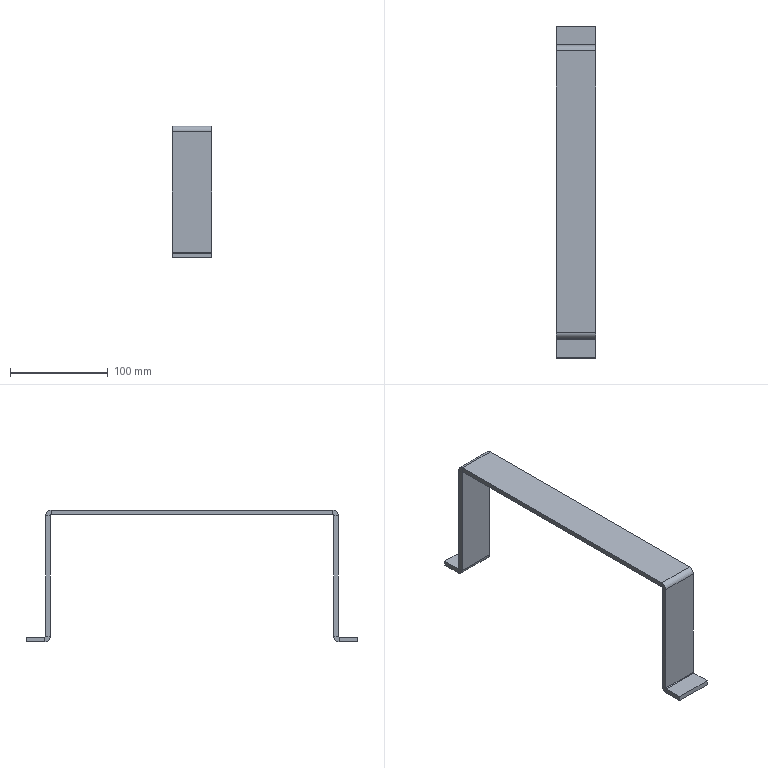Part | SolidWorks | features EdgeFlange 2, FlatPattern 1, SMBaseFlange 1, SheetMetal 1 | 1 solid | 38 faces | box 40 x 340 x 135 mm | volume 118889 mm3 | plane 30 | cylinder 8 | commonest cylinder face diameters 1.473 x4 11.473 x4
STEP:
#1=CARTESIAN_POINT('',(20.,-150.,-5.737));
#2=VERTEX_POINT('',#1);
#3=CARTESIAN_POINT('',(20.,-150.,-129.263));
#4=VERTEX_POINT('',#3);
#5=CARTESIAN_POINT('',(20.,-150.,-5.));
#6=DIRECTION('',(0.,0.,-1.));
#7=VECTOR('',#6,1000.);
#8=LINE('',#5,#7);
#9=EDGE_CURVE('',#2,#4,#8,.T.);
#10=ORIENTED_EDGE('',*,*,#9,.T.);
#11=CARTESIAN_POINT('',(20.,-145.,-129.263));
#12=VERTEX_POINT('',#11);
#13=CARTESIAN_POINT('',(20.,-150.,-129.263));
#14=DIRECTION('',(0.,1.,0.));
#15=VECTOR('',#14,1000.);
#16=LINE('',#13,#15);
#17=EDGE_CURVE('',#4,#12,#16,.T.);
#18=ORIENTED_EDGE('',*,*,#17,.T.);
#19=CARTESIAN_POINT('',(20.,-145.,-5.737));
#20=VERTEX_POINT('',#19);
#21=CARTESIAN_POINT('',(20.,-145.,0.));
#22=DIRECTION('',(0.,0.,-1.));
#23=VECTOR('',#22,1000.);
#24=LINE('',#21,#23);
#25=EDGE_CURVE('',#20,#12,#24,.T.);
#26=ORIENTED_EDGE('',*,*,#25,.F.);
#27=CARTESIAN_POINT('',(20.,-150.,-5.737));
#28=DIRECTION('',(0.,-1.,0.));
#29=VECTOR('',#28,1000.);
#30=LINE('',#27,#29);
#31=EDGE_CURVE('',#20,#2,#30,.T.);
#32=ORIENTED_EDGE('',*,*,#31,.T.);
#33=EDGE_LOOP('',(#10,#18,#26,#32));
#34=FACE_OUTER_BOUND('',#33,.T.);
#35=CARTESIAN_POINT('',(20.,-150.,-5.));
#36=DIRECTION('',(1.,0.,0.));
#37=DIRECTION('',(0.,0.,-1.));
#38=AXIS2_PLACEMENT_3D('',#35,#36,#37);
#39=PLANE('',#38);
#40=ADVANCED_FACE('',(#34),#39,.T.);
#41=CARTESIAN_POINT('',(-20.,-150.,-129.263));
#42=VERTEX_POINT('',#41);
#43=CARTESIAN_POINT('',(20.,-150.,-129.263));
#44=DIRECTION('',(-1.,0.,0.));
#45=VECTOR('',#44,1000.);
#46=LINE('',#43,#45);
#47=EDGE_CURVE('',#4,#42,#46,.T.);
#48=ORIENTED_EDGE('',*,*,#47,.F.);
#49=ORIENTED_EDGE('',*,*,#9,.F.);
#50=CARTESIAN_POINT('',(-20.,-150.,-5.737));
#51=VERTEX_POINT('',#50);
#52=CARTESIAN_POINT('',(20.,-150.,-5.737));
#53=DIRECTION('',(1.,0.,0.));
#54=VECTOR('',#53,1000.);
#55=LINE('',#52,#54);
#56=EDGE_CURVE('',#51,#2,#55,.T.);
#57=ORIENTED_EDGE('',*,*,#56,.F.);
#58=CARTESIAN_POINT('',(-20.,-150.,-135.));
#59=DIRECTION('',(0.,0.,1.));
#60=VECTOR('',#59,1000.);
#61=LINE('',#58,#60);
#62=EDGE_CURVE('',#42,#51,#61,.T.);
#63=ORIENTED_EDGE('',*,*,#62,.F.);
#64=EDGE_LOOP('',(#48,#49,#57,#63));
#65=FACE_OUTER_BOUND('',#64,.T.);
#66=CARTESIAN_POINT('',(0.,-150.,0.));
#67=DIRECTION('',(0.,1.,0.));
#68=DIRECTION('',(0.,0.,1.));
#69=AXIS2_PLACEMENT_3D('',#66,#67,#68);
#70=PLANE('',#69);
#71=ADVANCED_FACE('',(#65),#70,.F.);
#72=ORIENTED_EDGE('',*,*,#25,.T.);
#73=CARTESIAN_POINT('',(-20.,-145.,-129.263));
#74=VERTEX_POINT('',#73);
#75=CARTESIAN_POINT('',(20.,-145.,-129.263));
#76=DIRECTION('',(-1.,0.,0.));
#77=VECTOR('',#76,1000.);
#78=LINE('',#75,#77);
#79=EDGE_CURVE('',#12,#74,#78,.T.);
#80=ORIENTED_EDGE('',*,*,#79,.T.);
#81=CARTESIAN_POINT('',(-20.,-145.,-5.737));
#82=VERTEX_POINT('',#81);
#83=CARTESIAN_POINT('',(-20.,-145.,0.));
#84=DIRECTION('',(0.,0.,1.));
#85=VECTOR('',#84,1000.);
#86=LINE('',#83,#85);
#87=EDGE_CURVE('',#74,#82,#86,.T.);
#88=ORIENTED_EDGE('',*,*,#87,.T.);
#89=CARTESIAN_POINT('',(20.,-145.,-5.737));
#90=DIRECTION('',(-1.,0.,0.));
#91=VECTOR('',#90,1000.);
#92=LINE('',#89,#91);
#93=EDGE_CURVE('',#20,#82,#92,.T.);
#94=ORIENTED_EDGE('',*,*,#93,.F.);
#95=EDGE_LOOP('',(#72,#80,#88,#94));
#96=FACE_OUTER_BOUND('',#95,.T.);
#97=CARTESIAN_POINT('',(0.,-145.,0.));
#98=DIRECTION('',(0.,1.,0.));
#99=DIRECTION('',(0.,0.,1.));
#100=AXIS2_PLACEMENT_3D('',#97,#98,#99);
#101=PLANE('',#100);
#102=ADVANCED_FACE('',(#96),#101,.T.);
#103=CARTESIAN_POINT('',(-20.,150.,-5.737));
#104=VERTEX_POINT('',#103);
#105=CARTESIAN_POINT('',(-20.,150.,-129.263));
#106=VERTEX_POINT('',#105);
#107=CARTESIAN_POINT('',(-20.,150.,-135.));
#108=DIRECTION('',(0.,0.,-1.));
#109=VECTOR('',#108,1000.);
#110=LINE('',#107,#109);
#111=EDGE_CURVE('',#104,#106,#110,.T.);
#112=ORIENTED_EDGE('',*,*,#111,.T.);
#113=CARTESIAN_POINT('',(-20.,145.,-129.263));
#114=VERTEX_POINT('',#113);
#115=CARTESIAN_POINT('',(-20.,150.,-129.263));
#116=DIRECTION('',(0.,-1.,0.));
#117=VECTOR('',#116,1000.);
#118=LINE('',#115,#117);
#119=EDGE_CURVE('',#106,#114,#118,.T.);
#120=ORIENTED_EDGE('',*,*,#119,.T.);
#121=CARTESIAN_POINT('',(-20.,145.,-5.737));
#122=VERTEX_POINT('',#121);
#123=CARTESIAN_POINT('',(-20.,145.,0.));
#124=DIRECTION('',(0.,0.,-1.));
#125=VECTOR('',#124,1000.);
#126=LINE('',#123,#125);
#127=EDGE_CURVE('',#122,#114,#126,.T.);
#128=ORIENTED_EDGE('',*,*,#127,.F.);
#129=CARTESIAN_POINT('',(-20.,150.,-5.737));
#130=DIRECTION('',(0.,1.,0.));
#131=VECTOR('',#130,1000.);
#132=LINE('',#129,#131);
#133=EDGE_CURVE('',#122,#104,#132,.T.);
#134=ORIENTED_EDGE('',*,*,#133,.T.);
#135=EDGE_LOOP('',(#112,#120,#128,#134));
#136=FACE_OUTER_BOUND('',#135,.T.);
#137=CARTESIAN_POINT('',(-20.,150.,-135.));
#138=DIRECTION('',(-1.,0.,0.));
#139=DIRECTION('',(0.,0.,1.));
#140=AXIS2_PLACEMENT_3D('',#137,#138,#139);
#141=PLANE('',#140);
#142=ADVANCED_FACE('',(#136),#141,.T.);
#143=CARTESIAN_POINT('',(20.,150.,-129.263));
#144=VERTEX_POINT('',#143);
#145=CARTESIAN_POINT('',(20.,150.,-5.737));
#146=VERTEX_POINT('',#145);
#147=CARTESIAN_POINT('',(20.,150.,-5.));
#148=DIRECTION('',(0.,0.,1.));
#149=VECTOR('',#148,1000.);
#150=LINE('',#147,#149);
#151=EDGE_CURVE('',#144,#146,#150,.T.);
#152=ORIENTED_EDGE('',*,*,#151,.F.);
#153=CARTESIAN_POINT('',(-20.,150.,-129.263));
#154=DIRECTION('',(1.,0.,0.));
#155=VECTOR('',#154,1000.);
#156=LINE('',#153,#155);
#157=EDGE_CURVE('',#106,#144,#156,.T.);
#158=ORIENTED_EDGE('',*,*,#157,.F.);
#159=ORIENTED_EDGE('',*,*,#111,.F.);
#160=CARTESIAN_POINT('',(0.,150.,-5.737));
#161=DIRECTION('',(1.,0.,0.));
#162=VECTOR('',#161,1000.);
#163=LINE('',#160,#162);
#164=EDGE_CURVE('',#104,#146,#163,.T.);
#165=ORIENTED_EDGE('',*,*,#164,.T.);
#166=EDGE_LOOP('',(#152,#158,#159,#165));
#167=FACE_OUTER_BOUND('',#166,.T.);
#168=CARTESIAN_POINT('',(0.,150.,0.));
#169=DIRECTION('',(0.,1.,0.));
#170=DIRECTION('',(0.,0.,1.));
#171=AXIS2_PLACEMENT_3D('',#168,#169,#170);
#172=PLANE('',#171);
#173=ADVANCED_FACE('',(#167),#172,.T.);
#174=CARTESIAN_POINT('',(20.,145.,-129.263));
#175=VERTEX_POINT('',#174);
#176=CARTESIAN_POINT('',(-20.,145.,-129.263));
#177=DIRECTION('',(1.,0.,0.));
#178=VECTOR('',#177,1000.);
#179=LINE('',#176,#178);
#180=EDGE_CURVE('',#114,#175,#179,.T.);
#181=ORIENTED_EDGE('',*,*,#180,.T.);
#182=CARTESIAN_POINT('',(20.,145.,-5.737));
#183=VERTEX_POINT('',#182);
#184=CARTESIAN_POINT('',(20.,145.,0.));
#185=DIRECTION('',(0.,0.,1.));
#186=VECTOR('',#185,1000.);
#187=LINE('',#184,#186);
#188=EDGE_CURVE('',#175,#183,#187,.T.);
#189=ORIENTED_EDGE('',*,*,#188,.T.);
#190=CARTESIAN_POINT('',(-20.,145.,-5.737));
#191=DIRECTION('',(1.,0.,0.));
#192=VECTOR('',#191,1000.);
#193=LINE('',#190,#192);
#194=EDGE_CURVE('',#122,#183,#193,.T.);
#195=ORIENTED_EDGE('',*,*,#194,.F.);
#196=ORIENTED_EDGE('',*,*,#127,.T.);
#197=EDGE_LOOP('',(#181,#189,#195,#196));
#198=FACE_OUTER_BOUND('',#197,.T.);
#199=CARTESIAN_POINT('',(0.,145.,0.));
#200=DIRECTION('',(0.,1.,0.));
#201=DIRECTION('',(0.,0.,1.));
#202=AXIS2_PLACEMENT_3D('',#199,#200,#201);
#203=PLANE('',#202);
#204=ADVANCED_FACE('',(#198),#203,.F.);
#205=CARTESIAN_POINT('',(20.,-144.263,-5.));
#206=VERTEX_POINT('',#205);
#207=CARTESIAN_POINT('',(20.,144.263,-5.));
#208=VERTEX_POINT('',#207);
#209=CARTESIAN_POINT('',(20.,-150.,-5.));
#210=DIRECTION('',(0.,1.,0.));
#211=VECTOR('',#210,1000.);
#212=LINE('',#209,#211);
#213=EDGE_CURVE('',#206,#208,#212,.T.);
#214=ORIENTED_EDGE('',*,*,#213,.F.);
#215=CARTESIAN_POINT('',(-20.,-144.263,-5.));
#216=VERTEX_POINT('',#215);
#217=CARTESIAN_POINT('',(-20.,-144.263,-5.));
#218=DIRECTION('',(1.,0.,0.));
#219=VECTOR('',#218,1000.);
#220=LINE('',#217,#219);
#221=EDGE_CURVE('',#216,#206,#220,.T.);
#222=ORIENTED_EDGE('',*,*,#221,.F.);
#223=CARTESIAN_POINT('',(-20.,144.263,-5.));
#224=VERTEX_POINT('',#223);
#225=CARTESIAN_POINT('',(-20.,-150.,-5.));
#226=DIRECTION('',(0.,-1.,0.));
#227=VECTOR('',#226,1000.);
#228=LINE('',#225,#227);
#229=EDGE_CURVE('',#224,#216,#228,.T.);
#230=ORIENTED_EDGE('',*,*,#229,.F.);
#231=CARTESIAN_POINT('',(20.,144.263,-5.));
#232=DIRECTION('',(-1.,0.,0.));
#233=VECTOR('',#232,1000.);
#234=LINE('',#231,#233);
#235=EDGE_CURVE('',#208,#224,#234,.T.);
#236=ORIENTED_EDGE('',*,*,#235,.F.);
#237=EDGE_LOOP('',(#214,#222,#230,#236));
#238=FACE_OUTER_BOUND('',#237,.T.);
#239=CARTESIAN_POINT('',(0.,0.,-5.));
#240=DIRECTION('',(0.,0.,-1.));
#241=DIRECTION('',(-1.,0.,0.));
#242=AXIS2_PLACEMENT_3D('',#239,#240,#241);
#243=PLANE('',#242);
#244=ADVANCED_FACE('',(#238),#243,.T.);
#245=CARTESIAN_POINT('',(-20.,-144.263,0.));
#246=VERTEX_POINT('',#245);
#247=CARTESIAN_POINT('',(20.,-144.263,0.));
#248=VERTEX_POINT('',#247);
#249=CARTESIAN_POINT('',(-20.,-144.263,0.));
#250=DIRECTION('',(1.,0.,0.));
#251=VECTOR('',#250,1000.);
#252=LINE('',#249,#251);
#253=EDGE_CURVE('',#246,#248,#252,.T.);
#254=ORIENTED_EDGE('',*,*,#253,.T.);
#255=CARTESIAN_POINT('',(20.,144.263,0.));
#256=VERTEX_POINT('',#255);
#257=CARTESIAN_POINT('',(20.,-150.,0.));
#258=DIRECTION('',(0.,1.,0.));
#259=VECTOR('',#258,1000.);
#260=LINE('',#257,#259);
#261=EDGE_CURVE('',#248,#256,#260,.T.);
#262=ORIENTED_EDGE('',*,*,#261,.T.);
#263=CARTESIAN_POINT('',(-20.,144.263,0.));
#264=VERTEX_POINT('',#263);
#265=CARTESIAN_POINT('',(20.,144.263,0.));
#266=DIRECTION('',(-1.,0.,0.));
#267=VECTOR('',#266,1000.);
#268=LINE('',#265,#267);
#269=EDGE_CURVE('',#256,#264,#268,.T.);
#270=ORIENTED_EDGE('',*,*,#269,.T.);
#271=CARTESIAN_POINT('',(-20.,-150.,0.));
#272=DIRECTION('',(0.,-1.,0.));
#273=VECTOR('',#272,1000.);
#274=LINE('',#271,#273);
#275=EDGE_CURVE('',#264,#246,#274,.T.);
#276=ORIENTED_EDGE('',*,*,#275,.T.);
#277=EDGE_LOOP('',(#254,#262,#270,#276));
#278=FACE_OUTER_BOUND('',#277,.T.);
#279=CARTESIAN_POINT('',(0.,0.,0.));
#280=DIRECTION('',(0.,0.,-1.));
#281=DIRECTION('',(-1.,0.,0.));
#282=AXIS2_PLACEMENT_3D('',#279,#280,#281);
#283=PLANE('',#282);
#284=ADVANCED_FACE('',(#278),#283,.F.);
#285=ORIENTED_EDGE('',*,*,#229,.T.);
#286=CARTESIAN_POINT('',(-20.,-144.263,-5.));
#287=DIRECTION('',(0.,0.,1.));
#288=VECTOR('',#287,1000.);
#289=LINE('',#286,#288);
#290=EDGE_CURVE('',#216,#246,#289,.T.);
#291=ORIENTED_EDGE('',*,*,#290,.T.);
#292=ORIENTED_EDGE('',*,*,#275,.F.);
#293=CARTESIAN_POINT('',(-20.,144.263,-5.));
#294=DIRECTION('',(0.,0.,1.));
#295=VECTOR('',#294,1000.);
#296=LINE('',#293,#295);
#297=EDGE_CURVE('',#224,#264,#296,.T.);
#298=ORIENTED_EDGE('',*,*,#297,.F.);
#299=EDGE_LOOP('',(#285,#291,#292,#298));
#300=FACE_OUTER_BOUND('',#299,.T.);
#301=CARTESIAN_POINT('',(-20.,-150.,-5.));
#302=DIRECTION('',(-1.,0.,0.));
#303=DIRECTION('',(0.,0.,1.));
#304=AXIS2_PLACEMENT_3D('',#301,#302,#303);
#305=PLANE('',#304);
#306=ADVANCED_FACE('',(#300),#305,.T.);
#307=CARTESIAN_POINT('',(20.,-144.263,-5.));
#308=DIRECTION('',(0.,0.,1.));
#309=VECTOR('',#308,1000.);
#310=LINE('',#307,#309);
#311=EDGE_CURVE('',#206,#248,#310,.T.);
#312=ORIENTED_EDGE('',*,*,#311,.F.);
#313=ORIENTED_EDGE('',*,*,#213,.T.);
#314=CARTESIAN_POINT('',(20.,144.263,-5.));
#315=DIRECTION('',(0.,0.,1.));
#316=VECTOR('',#315,1000.);
#317=LINE('',#314,#316);
#318=EDGE_CURVE('',#208,#256,#317,.T.);
#319=ORIENTED_EDGE('',*,*,#318,.T.);
#320=ORIENTED_EDGE('',*,*,#261,.F.);
#321=EDGE_LOOP('',(#312,#313,#319,#320));
#322=FACE_OUTER_BOUND('',#321,.T.);
#323=CARTESIAN_POINT('',(20.,-150.,-5.));
#324=DIRECTION('',(1.,0.,0.));
#325=DIRECTION('',(0.,0.,-1.));
#326=AXIS2_PLACEMENT_3D('',#323,#324,#325);
#327=PLANE('',#326);
#328=ADVANCED_FACE('',(#322),#327,.T.);
#329=ORIENTED_EDGE('',*,*,#133,.F.);
#330=CARTESIAN_POINT('',(-20.,144.263,-5.737));
#331=DIRECTION('',(-1.,0.,0.));
#332=DIRECTION('',(0.,0.,-1.));
#333=AXIS2_PLACEMENT_3D('',#330,#331,#332);
#334=CIRCLE('',#333,0.7366);
#335=EDGE_CURVE('',#224,#122,#334,.T.);
#336=ORIENTED_EDGE('',*,*,#335,.F.);
#337=ORIENTED_EDGE('',*,*,#297,.T.);
#338=CARTESIAN_POINT('',(-20.,144.263,-5.737));
#339=DIRECTION('',(-1.,0.,0.));
#340=DIRECTION('',(0.,0.,-1.));
#341=AXIS2_PLACEMENT_3D('',#338,#339,#340);
#342=CIRCLE('',#341,5.737);
#343=EDGE_CURVE('',#264,#104,#342,.T.);
#344=ORIENTED_EDGE('',*,*,#343,.T.);
#345=EDGE_LOOP('',(#329,#336,#337,#344));
#346=FACE_OUTER_BOUND('',#345,.T.);
#347=CARTESIAN_POINT('',(-20.,144.263,-5.737));
#348=DIRECTION('',(-1.,0.,0.));
#349=DIRECTION('',(0.,0.,1.));
#350=AXIS2_PLACEMENT_3D('',#347,#348,#349);
#351=PLANE('',#350);
#352=ADVANCED_FACE('',(#346),#351,.T.);
#353=CARTESIAN_POINT('',(20.,144.263,-5.737));
#354=DIRECTION('',(1.,0.,0.));
#355=DIRECTION('',(0.,0.,-1.));
#356=AXIS2_PLACEMENT_3D('',#353,#354,#355);
#357=CIRCLE('',#356,0.7366);
#358=EDGE_CURVE('',#183,#208,#357,.T.);
#359=ORIENTED_EDGE('',*,*,#358,.F.);
#360=CARTESIAN_POINT('',(20.,145.,-5.737));
#361=DIRECTION('',(0.,1.,0.));
#362=VECTOR('',#361,1000.);
#363=LINE('',#360,#362);
#364=EDGE_CURVE('',#183,#146,#363,.T.);
#365=ORIENTED_EDGE('',*,*,#364,.T.);
#366=CARTESIAN_POINT('',(20.,144.263,-5.737));
#367=DIRECTION('',(1.,0.,0.));
#368=DIRECTION('',(0.,0.,-1.));
#369=AXIS2_PLACEMENT_3D('',#366,#367,#368);
#370=CIRCLE('',#369,5.737);
#371=EDGE_CURVE('',#146,#256,#370,.T.);
#372=ORIENTED_EDGE('',*,*,#371,.T.);
#373=ORIENTED_EDGE('',*,*,#318,.F.);
#374=EDGE_LOOP('',(#359,#365,#372,#373));
#375=FACE_OUTER_BOUND('',#374,.T.);
#376=CARTESIAN_POINT('',(20.,144.263,-5.737));
#377=DIRECTION('',(-1.,0.,0.));
#378=DIRECTION('',(0.,0.,1.));
#379=AXIS2_PLACEMENT_3D('',#376,#377,#378);
#380=PLANE('',#379);
#381=ADVANCED_FACE('',(#375),#380,.F.);
#382=ORIENTED_EDGE('',*,*,#269,.F.);
#383=ORIENTED_EDGE('',*,*,#371,.F.);
#384=ORIENTED_EDGE('',*,*,#164,.F.);
#385=ORIENTED_EDGE('',*,*,#343,.F.);
#386=EDGE_LOOP('',(#382,#383,#384,#385));
#387=FACE_OUTER_BOUND('',#386,.T.);
#388=CARTESIAN_POINT('',(20.,144.263,-5.737));
#389=DIRECTION('',(1.,0.,0.));
#390=DIRECTION('',(0.,1.,0.));
#391=AXIS2_PLACEMENT_3D('',#388,#389,#390);
#392=CYLINDRICAL_SURFACE('',#391,5.737);
#393=ADVANCED_FACE('',(#387),#392,.T.);
#394=ORIENTED_EDGE('',*,*,#235,.T.);
#395=ORIENTED_EDGE('',*,*,#335,.T.);
#396=ORIENTED_EDGE('',*,*,#194,.T.);
#397=ORIENTED_EDGE('',*,*,#358,.T.);
#398=EDGE_LOOP('',(#394,#395,#396,#397));
#399=FACE_OUTER_BOUND('',#398,.T.);
#400=CARTESIAN_POINT('',(20.,144.263,-5.737));
#401=DIRECTION('',(1.,0.,0.));
#402=DIRECTION('',(0.,1.,0.));
#403=AXIS2_PLACEMENT_3D('',#400,#401,#402);
#404=CYLINDRICAL_SURFACE('',#403,0.7366);
#405=ADVANCED_FACE('',(#399),#404,.F.);
#406=CARTESIAN_POINT('',(20.,150.,-129.263));
#407=DIRECTION('',(0.,-1.,0.));
#408=VECTOR('',#407,1000.);
#409=LINE('',#406,#408);
#410=EDGE_CURVE('',#144,#175,#409,.T.);
#411=ORIENTED_EDGE('',*,*,#410,.F.);
#412=ORIENTED_EDGE('',*,*,#151,.T.);
#413=ORIENTED_EDGE('',*,*,#364,.F.);
#414=ORIENTED_EDGE('',*,*,#188,.F.);
#415=EDGE_LOOP('',(#411,#412,#413,#414));
#416=FACE_OUTER_BOUND('',#415,.T.);
#417=CARTESIAN_POINT('',(20.,150.,-5.));
#418=DIRECTION('',(1.,0.,0.));
#419=DIRECTION('',(0.,0.,-1.));
#420=AXIS2_PLACEMENT_3D('',#417,#418,#419);
#421=PLANE('',#420);
#422=ADVANCED_FACE('',(#416),#421,.T.);
#423=ORIENTED_EDGE('',*,*,#31,.F.);
#424=CARTESIAN_POINT('',(20.,-144.263,-5.737));
#425=DIRECTION('',(1.,0.,0.));
#426=DIRECTION('',(0.,0.,1.));
#427=AXIS2_PLACEMENT_3D('',#424,#425,#426);
#428=CIRCLE('',#427,0.7366);
#429=EDGE_CURVE('',#206,#20,#428,.T.);
#430=ORIENTED_EDGE('',*,*,#429,.F.);
#431=ORIENTED_EDGE('',*,*,#311,.T.);
#432=CARTESIAN_POINT('',(20.,-144.263,-5.737));
#433=DIRECTION('',(1.,0.,0.));
#434=DIRECTION('',(0.,0.,1.));
#435=AXIS2_PLACEMENT_3D('',#432,#433,#434);
#436=CIRCLE('',#435,5.737);
#437=EDGE_CURVE('',#248,#2,#436,.T.);
#438=ORIENTED_EDGE('',*,*,#437,.T.);
#439=EDGE_LOOP('',(#423,#430,#431,#438));
#440=FACE_OUTER_BOUND('',#439,.T.);
#441=CARTESIAN_POINT('',(20.,-144.263,-5.737));
#442=DIRECTION('',(1.,0.,0.));
#443=DIRECTION('',(0.,0.,-1.));
#444=AXIS2_PLACEMENT_3D('',#441,#442,#443);
#445=PLANE('',#444);
#446=ADVANCED_FACE('',(#440),#445,.T.);
#447=CARTESIAN_POINT('',(-20.,-144.263,-5.737));
#448=DIRECTION('',(-1.,0.,0.));
#449=DIRECTION('',(0.,0.,1.));
#450=AXIS2_PLACEMENT_3D('',#447,#448,#449);
#451=CIRCLE('',#450,0.7366);
#452=EDGE_CURVE('',#82,#216,#451,.T.);
#453=ORIENTED_EDGE('',*,*,#452,.F.);
#454=CARTESIAN_POINT('',(-20.,-145.,-5.737));
#455=DIRECTION('',(0.,-1.,0.));
#456=VECTOR('',#455,1000.);
#457=LINE('',#454,#456);
#458=EDGE_CURVE('',#82,#51,#457,.T.);
#459=ORIENTED_EDGE('',*,*,#458,.T.);
#460=CARTESIAN_POINT('',(-20.,-144.263,-5.737));
#461=DIRECTION('',(-1.,0.,0.));
#462=DIRECTION('',(0.,0.,1.));
#463=AXIS2_PLACEMENT_3D('',#460,#461,#462);
#464=CIRCLE('',#463,5.737);
#465=EDGE_CURVE('',#51,#246,#464,.T.);
#466=ORIENTED_EDGE('',*,*,#465,.T.);
#467=ORIENTED_EDGE('',*,*,#290,.F.);
#468=EDGE_LOOP('',(#453,#459,#466,#467));
#469=FACE_OUTER_BOUND('',#468,.T.);
#470=CARTESIAN_POINT('',(-20.,-144.263,-5.737));
#471=DIRECTION('',(1.,0.,0.));
#472=DIRECTION('',(0.,0.,-1.));
#473=AXIS2_PLACEMENT_3D('',#470,#471,#472);
#474=PLANE('',#473);
#475=ADVANCED_FACE('',(#469),#474,.F.);
#476=ORIENTED_EDGE('',*,*,#253,.F.);
#477=ORIENTED_EDGE('',*,*,#465,.F.);
#478=ORIENTED_EDGE('',*,*,#56,.T.);
#479=ORIENTED_EDGE('',*,*,#437,.F.);
#480=EDGE_LOOP('',(#476,#477,#478,#479));
#481=FACE_OUTER_BOUND('',#480,.T.);
#482=CARTESIAN_POINT('',(-20.,-144.263,-5.737));
#483=DIRECTION('',(-1.,0.,0.));
#484=DIRECTION('',(0.,-1.,0.));
#485=AXIS2_PLACEMENT_3D('',#482,#483,#484);
#486=CYLINDRICAL_SURFACE('',#485,5.737);
#487=ADVANCED_FACE('',(#481),#486,.T.);
#488=ORIENTED_EDGE('',*,*,#221,.T.);
#489=ORIENTED_EDGE('',*,*,#429,.T.);
#490=ORIENTED_EDGE('',*,*,#93,.T.);
#491=ORIENTED_EDGE('',*,*,#452,.T.);
#492=EDGE_LOOP('',(#488,#489,#490,#491));
#493=FACE_OUTER_BOUND('',#492,.T.);
#494=CARTESIAN_POINT('',(-20.,-144.263,-5.737));
#495=DIRECTION('',(-1.,0.,0.));
#496=DIRECTION('',(0.,-1.,0.));
#497=AXIS2_PLACEMENT_3D('',#494,#495,#496);
#498=CYLINDRICAL_SURFACE('',#497,0.7366);
#499=ADVANCED_FACE('',(#493),#498,.F.);
#500=CARTESIAN_POINT('',(-20.,-150.,-129.263));
#501=DIRECTION('',(0.,1.,0.));
#502=VECTOR('',#501,1000.);
#503=LINE('',#500,#502);
#504=EDGE_CURVE('',#42,#74,#503,.T.);
#505=ORIENTED_EDGE('',*,*,#504,.F.);
#506=ORIENTED_EDGE('',*,*,#62,.T.);
#507=ORIENTED_EDGE('',*,*,#458,.F.);
#508=ORIENTED_EDGE('',*,*,#87,.F.);
#509=EDGE_LOOP('',(#505,#506,#507,#508));
#510=FACE_OUTER_BOUND('',#509,.T.);
#511=CARTESIAN_POINT('',(-20.,-150.,-135.));
#512=DIRECTION('',(-1.,0.,0.));
#513=DIRECTION('',(0.,0.,1.));
#514=AXIS2_PLACEMENT_3D('',#511,#512,#513);
#515=PLANE('',#514);
#516=ADVANCED_FACE('',(#510),#515,.T.);
#517=CARTESIAN_POINT('',(20.,150.737,-130.));
#518=VERTEX_POINT('',#517);
#519=CARTESIAN_POINT('',(20.,150.737,-135.));
#520=VERTEX_POINT('',#519);
#521=CARTESIAN_POINT('',(20.,150.737,-135.));
#522=DIRECTION('',(0.,0.,-1.));
#523=VECTOR('',#522,1000.);
#524=LINE('',#521,#523);
#525=EDGE_CURVE('',#518,#520,#524,.T.);
#526=ORIENTED_EDGE('',*,*,#525,.F.);
#527=CARTESIAN_POINT('',(20.,150.737,-129.263));
#528=DIRECTION('',(1.,0.,0.));
#529=DIRECTION('',(0.,0.,1.));
#530=AXIS2_PLACEMENT_3D('',#527,#528,#529);
#531=CIRCLE('',#530,0.7366);
#532=EDGE_CURVE('',#144,#518,#531,.T.);
#533=ORIENTED_EDGE('',*,*,#532,.F.);
#534=ORIENTED_EDGE('',*,*,#410,.T.);
#535=CARTESIAN_POINT('',(20.,150.737,-129.263));
#536=DIRECTION('',(1.,0.,0.));
#537=DIRECTION('',(0.,0.,1.));
#538=AXIS2_PLACEMENT_3D('',#535,#536,#537);
#539=CIRCLE('',#538,5.737);
#540=EDGE_CURVE('',#175,#520,#539,.T.);
#541=ORIENTED_EDGE('',*,*,#540,.T.);
#542=EDGE_LOOP('',(#526,#533,#534,#541));
#543=FACE_OUTER_BOUND('',#542,.T.);
#544=CARTESIAN_POINT('',(20.,150.737,-129.263));
#545=DIRECTION('',(1.,0.,0.));
#546=DIRECTION('',(0.,0.,-1.));
#547=AXIS2_PLACEMENT_3D('',#544,#545,#546);
#548=PLANE('',#547);
#549=ADVANCED_FACE('',(#543),#548,.T.);
#550=CARTESIAN_POINT('',(-20.,150.737,-130.));
#551=VERTEX_POINT('',#550);
#552=CARTESIAN_POINT('',(-20.,150.737,-129.263));
#553=DIRECTION('',(-1.,0.,0.));
#554=DIRECTION('',(0.,0.,1.));
#555=AXIS2_PLACEMENT_3D('',#552,#553,#554);
#556=CIRCLE('',#555,0.7366);
#557=EDGE_CURVE('',#551,#106,#556,.T.);
#558=ORIENTED_EDGE('',*,*,#557,.F.);
#559=CARTESIAN_POINT('',(-20.,150.737,-135.));
#560=VERTEX_POINT('',#559);
#561=CARTESIAN_POINT('',(-20.,150.737,-130.));
#562=DIRECTION('',(0.,0.,-1.));
#563=VECTOR('',#562,1000.);
#564=LINE('',#561,#563);
#565=EDGE_CURVE('',#551,#560,#564,.T.);
#566=ORIENTED_EDGE('',*,*,#565,.T.);
#567=CARTESIAN_POINT('',(-20.,150.737,-129.263));
#568=DIRECTION('',(-1.,0.,0.));
#569=DIRECTION('',(0.,0.,1.));
#570=AXIS2_PLACEMENT_3D('',#567,#568,#569);
#571=CIRCLE('',#570,5.737);
#572=EDGE_CURVE('',#560,#114,#571,.T.);
#573=ORIENTED_EDGE('',*,*,#572,.T.);
#574=ORIENTED_EDGE('',*,*,#119,.F.);
#575=EDGE_LOOP('',(#558,#566,#573,#574));
#576=FACE_OUTER_BOUND('',#575,.T.);
#577=CARTESIAN_POINT('',(-20.,150.737,-129.263));
#578=DIRECTION('',(1.,0.,0.));
#579=DIRECTION('',(0.,0.,-1.));
#580=AXIS2_PLACEMENT_3D('',#577,#578,#579);
#581=PLANE('',#580);
#582=ADVANCED_FACE('',(#576),#581,.F.);
#583=ORIENTED_EDGE('',*,*,#180,.F.);
#584=ORIENTED_EDGE('',*,*,#572,.F.);
#585=CARTESIAN_POINT('',(20.,150.737,-135.));
#586=DIRECTION('',(1.,0.,0.));
#587=VECTOR('',#586,1000.);
#588=LINE('',#585,#587);
#589=EDGE_CURVE('',#560,#520,#588,.T.);
#590=ORIENTED_EDGE('',*,*,#589,.T.);
#591=ORIENTED_EDGE('',*,*,#540,.F.);
#592=EDGE_LOOP('',(#583,#584,#590,#591));
#593=FACE_OUTER_BOUND('',#592,.T.);
#594=CARTESIAN_POINT('',(-20.,150.737,-129.263));
#595=DIRECTION('',(-1.,0.,0.));
#596=DIRECTION('',(0.,0.,-1.));
#597=AXIS2_PLACEMENT_3D('',#594,#595,#596);
#598=CYLINDRICAL_SURFACE('',#597,5.737);
#599=ADVANCED_FACE('',(#593),#598,.T.);
#600=ORIENTED_EDGE('',*,*,#157,.T.);
#601=ORIENTED_EDGE('',*,*,#532,.T.);
#602=CARTESIAN_POINT('',(20.,150.737,-130.));
#603=DIRECTION('',(-1.,0.,0.));
#604=VECTOR('',#603,1000.);
#605=LINE('',#602,#604);
#606=EDGE_CURVE('',#518,#551,#605,.T.);
#607=ORIENTED_EDGE('',*,*,#606,.T.);
#608=ORIENTED_EDGE('',*,*,#557,.T.);
#609=EDGE_LOOP('',(#600,#601,#607,#608));
#610=FACE_OUTER_BOUND('',#609,.T.);
#611=CARTESIAN_POINT('',(-20.,150.737,-129.263));
#612=DIRECTION('',(-1.,0.,0.));
#613=DIRECTION('',(0.,0.,-1.));
#614=AXIS2_PLACEMENT_3D('',#611,#612,#613);
#615=CYLINDRICAL_SURFACE('',#614,0.7366);
#616=ADVANCED_FACE('',(#610),#615,.F.);
#617=ORIENTED_EDGE('',*,*,#565,.F.);
#618=CARTESIAN_POINT('',(-20.,170.,-130.));
#619=VERTEX_POINT('',#618);
#620=CARTESIAN_POINT('',(-20.,170.,-130.));
#621=DIRECTION('',(0.,1.,0.));
#622=VECTOR('',#621,1000.);
#623=LINE('',#620,#622);
#624=EDGE_CURVE('',#551,#619,#623,.T.);
#625=ORIENTED_EDGE('',*,*,#624,.T.);
#626=CARTESIAN_POINT('',(-20.,170.,-135.));
#627=VERTEX_POINT('',#626);
#628=CARTESIAN_POINT('',(-20.,170.,-135.));
#629=DIRECTION('',(0.,0.,1.));
#630=VECTOR('',#629,1000.);
#631=LINE('',#628,#630);
#632=EDGE_CURVE('',#627,#619,#631,.T.);
#633=ORIENTED_EDGE('',*,*,#632,.F.);
#634=CARTESIAN_POINT('',(-20.,0.,-135.));
#635=DIRECTION('',(0.,1.,0.));
#636=VECTOR('',#635,1000.);
#637=LINE('',#634,#636);
#638=EDGE_CURVE('',#560,#627,#637,.T.);
#639=ORIENTED_EDGE('',*,*,#638,.F.);
#640=EDGE_LOOP('',(#617,#625,#633,#639));
#641=FACE_OUTER_BOUND('',#640,.T.);
#642=CARTESIAN_POINT('',(-20.,170.,-135.));
#643=DIRECTION('',(1.,0.,0.));
#644=DIRECTION('',(0.,0.,-1.));
#645=AXIS2_PLACEMENT_3D('',#642,#643,#644);
#646=PLANE('',#645);
#647=ADVANCED_FACE('',(#641),#646,.F.);
#648=ORIENTED_EDGE('',*,*,#525,.T.);
#649=CARTESIAN_POINT('',(20.,170.,-135.));
#650=VERTEX_POINT('',#649);
#651=CARTESIAN_POINT('',(20.,0.,-135.));
#652=DIRECTION('',(0.,-1.,0.));
#653=VECTOR('',#652,1000.);
#654=LINE('',#651,#653);
#655=EDGE_CURVE('',#650,#520,#654,.T.);
#656=ORIENTED_EDGE('',*,*,#655,.F.);
#657=CARTESIAN_POINT('',(20.,170.,-130.));
#658=VERTEX_POINT('',#657);
#659=CARTESIAN_POINT('',(20.,170.,-135.));
#660=DIRECTION('',(0.,0.,1.));
#661=VECTOR('',#660,1000.);
#662=LINE('',#659,#661);
#663=EDGE_CURVE('',#650,#658,#662,.T.);
#664=ORIENTED_EDGE('',*,*,#663,.T.);
#665=CARTESIAN_POINT('',(20.,150.,-130.));
#666=DIRECTION('',(0.,-1.,0.));
#667=VECTOR('',#666,1000.);
#668=LINE('',#665,#667);
#669=EDGE_CURVE('',#658,#518,#668,.T.);
#670=ORIENTED_EDGE('',*,*,#669,.T.);
#671=EDGE_LOOP('',(#648,#656,#664,#670));
#672=FACE_OUTER_BOUND('',#671,.T.);
#673=CARTESIAN_POINT('',(20.,150.,-135.));
#674=DIRECTION('',(-1.,0.,0.));
#675=DIRECTION('',(0.,0.,1.));
#676=AXIS2_PLACEMENT_3D('',#673,#674,#675);
#677=PLANE('',#676);
#678=ADVANCED_FACE('',(#672),#677,.F.);
#679=ORIENTED_EDGE('',*,*,#589,.F.);
#680=ORIENTED_EDGE('',*,*,#638,.T.);
#681=CARTESIAN_POINT('',(0.,170.,-135.));
#682=DIRECTION('',(1.,0.,0.));
#683=VECTOR('',#682,1000.);
#684=LINE('',#681,#683);
#685=EDGE_CURVE('',#627,#650,#684,.T.);
#686=ORIENTED_EDGE('',*,*,#685,.T.);
#687=ORIENTED_EDGE('',*,*,#655,.T.);
#688=EDGE_LOOP('',(#679,#680,#686,#687));
#689=FACE_OUTER_BOUND('',#688,.T.);
#690=CARTESIAN_POINT('',(0.,0.,-135.));
#691=DIRECTION('',(0.,0.,1.));
#692=DIRECTION('',(1.,0.,0.));
#693=AXIS2_PLACEMENT_3D('',#690,#691,#692);
#694=PLANE('',#693);
#695=ADVANCED_FACE('',(#689),#694,.F.);
#696=ORIENTED_EDGE('',*,*,#624,.F.);
#697=ORIENTED_EDGE('',*,*,#606,.F.);
#698=ORIENTED_EDGE('',*,*,#669,.F.);
#699=CARTESIAN_POINT('',(20.,170.,-130.));
#700=DIRECTION('',(1.,0.,0.));
#701=VECTOR('',#700,1000.);
#702=LINE('',#699,#701);
#703=EDGE_CURVE('',#619,#658,#702,.T.);
#704=ORIENTED_EDGE('',*,*,#703,.F.);
#705=EDGE_LOOP('',(#696,#697,#698,#704));
#706=FACE_OUTER_BOUND('',#705,.T.);
#707=CARTESIAN_POINT('',(0.,0.,-130.));
#708=DIRECTION('',(0.,0.,1.));
#709=DIRECTION('',(1.,0.,0.));
#710=AXIS2_PLACEMENT_3D('',#707,#708,#709);
#711=PLANE('',#710);
#712=ADVANCED_FACE('',(#706),#711,.T.);
#713=ORIENTED_EDGE('',*,*,#703,.T.);
#714=ORIENTED_EDGE('',*,*,#663,.F.);
#715=ORIENTED_EDGE('',*,*,#685,.F.);
#716=ORIENTED_EDGE('',*,*,#632,.T.);
#717=EDGE_LOOP('',(#713,#714,#715,#716));
#718=FACE_OUTER_BOUND('',#717,.T.);
#719=CARTESIAN_POINT('',(20.,170.,-135.));
#720=DIRECTION('',(0.,-1.,0.));
#721=DIRECTION('',(0.,0.,-1.));
#722=AXIS2_PLACEMENT_3D('',#719,#720,#721);
#723=PLANE('',#722);
#724=ADVANCED_FACE('',(#718),#723,.F.);
#725=CARTESIAN_POINT('',(-20.,-150.737,-130.));
#726=VERTEX_POINT('',#725);
#727=CARTESIAN_POINT('',(-20.,-150.737,-135.));
#728=VERTEX_POINT('',#727);
#729=CARTESIAN_POINT('',(-20.,-150.737,-135.));
#730=DIRECTION('',(0.,0.,-1.));
#731=VECTOR('',#730,1000.);
#732=LINE('',#729,#731);
#733=EDGE_CURVE('',#726,#728,#732,.T.);
#734=ORIENTED_EDGE('',*,*,#733,.F.);
#735=CARTESIAN_POINT('',(-20.,-150.737,-129.263));
#736=DIRECTION('',(-1.,0.,0.));
#737=DIRECTION('',(0.,0.,-1.));
#738=AXIS2_PLACEMENT_3D('',#735,#736,#737);
#739=CIRCLE('',#738,0.7366);
#740=EDGE_CURVE('',#42,#726,#739,.T.);
#741=ORIENTED_EDGE('',*,*,#740,.F.);
#742=ORIENTED_EDGE('',*,*,#504,.T.);
#743=CARTESIAN_POINT('',(-20.,-150.737,-129.263));
#744=DIRECTION('',(-1.,0.,0.));
#745=DIRECTION('',(0.,0.,-1.));
#746=AXIS2_PLACEMENT_3D('',#743,#744,#745);
#747=CIRCLE('',#746,5.737);
#748=EDGE_CURVE('',#74,#728,#747,.T.);
#749=ORIENTED_EDGE('',*,*,#748,.T.);
#750=EDGE_LOOP('',(#734,#741,#742,#749));
#751=FACE_OUTER_BOUND('',#750,.T.);
#752=CARTESIAN_POINT('',(-20.,-150.737,-129.263));
#753=DIRECTION('',(-1.,0.,0.));
#754=DIRECTION('',(0.,0.,1.));
#755=AXIS2_PLACEMENT_3D('',#752,#753,#754);
#756=PLANE('',#755);
#757=ADVANCED_FACE('',(#751),#756,.T.);
#758=CARTESIAN_POINT('',(20.,-150.737,-130.));
#759=VERTEX_POINT('',#758);
#760=CARTESIAN_POINT('',(20.,-150.737,-129.263));
#761=DIRECTION('',(1.,0.,0.));
#762=DIRECTION('',(0.,0.,-1.));
#763=AXIS2_PLACEMENT_3D('',#760,#761,#762);
#764=CIRCLE('',#763,0.7366);
#765=EDGE_CURVE('',#759,#4,#764,.T.);
#766=ORIENTED_EDGE('',*,*,#765,.F.);
#767=CARTESIAN_POINT('',(20.,-150.737,-135.));
#768=VERTEX_POINT('',#767);
#769=CARTESIAN_POINT('',(20.,-150.737,-130.));
#770=DIRECTION('',(0.,0.,-1.));
#771=VECTOR('',#770,1000.);
#772=LINE('',#769,#771);
#773=EDGE_CURVE('',#759,#768,#772,.T.);
#774=ORIENTED_EDGE('',*,*,#773,.T.);
#775=CARTESIAN_POINT('',(20.,-150.737,-129.263));
#776=DIRECTION('',(1.,0.,0.));
#777=DIRECTION('',(0.,0.,-1.));
#778=AXIS2_PLACEMENT_3D('',#775,#776,#777);
#779=CIRCLE('',#778,5.737);
#780=EDGE_CURVE('',#768,#12,#779,.T.);
#781=ORIENTED_EDGE('',*,*,#780,.T.);
#782=ORIENTED_EDGE('',*,*,#17,.F.);
#783=EDGE_LOOP('',(#766,#774,#781,#782));
#784=FACE_OUTER_BOUND('',#783,.T.);
#785=CARTESIAN_POINT('',(20.,-150.737,-129.263));
#786=DIRECTION('',(-1.,0.,0.));
#787=DIRECTION('',(0.,0.,1.));
#788=AXIS2_PLACEMENT_3D('',#785,#786,#787);
#789=PLANE('',#788);
#790=ADVANCED_FACE('',(#784),#789,.F.);
#791=ORIENTED_EDGE('',*,*,#79,.F.);
#792=ORIENTED_EDGE('',*,*,#780,.F.);
#793=CARTESIAN_POINT('',(-20.,-150.737,-135.));
#794=DIRECTION('',(-1.,0.,0.));
#795=VECTOR('',#794,1000.);
#796=LINE('',#793,#795);
#797=EDGE_CURVE('',#768,#728,#796,.T.);
#798=ORIENTED_EDGE('',*,*,#797,.T.);
#799=ORIENTED_EDGE('',*,*,#748,.F.);
#800=EDGE_LOOP('',(#791,#792,#798,#799));
#801=FACE_OUTER_BOUND('',#800,.T.);
#802=CARTESIAN_POINT('',(20.,-150.737,-129.263));
#803=DIRECTION('',(1.,0.,0.));
#804=DIRECTION('',(0.,0.,-1.));
#805=AXIS2_PLACEMENT_3D('',#802,#803,#804);
#806=CYLINDRICAL_SURFACE('',#805,5.737);
#807=ADVANCED_FACE('',(#801),#806,.T.);
#808=ORIENTED_EDGE('',*,*,#47,.T.);
#809=ORIENTED_EDGE('',*,*,#740,.T.);
#810=CARTESIAN_POINT('',(-20.,-150.737,-130.));
#811=DIRECTION('',(1.,0.,0.));
#812=VECTOR('',#811,1000.);
#813=LINE('',#810,#812);
#814=EDGE_CURVE('',#726,#759,#813,.T.);
#815=ORIENTED_EDGE('',*,*,#814,.T.);
#816=ORIENTED_EDGE('',*,*,#765,.T.);
#817=EDGE_LOOP('',(#808,#809,#815,#816));
#818=FACE_OUTER_BOUND('',#817,.T.);
#819=CARTESIAN_POINT('',(20.,-150.737,-129.263));
#820=DIRECTION('',(1.,0.,0.));
#821=DIRECTION('',(0.,0.,-1.));
#822=AXIS2_PLACEMENT_3D('',#819,#820,#821);
#823=CYLINDRICAL_SURFACE('',#822,0.7366);
#824=ADVANCED_FACE('',(#818),#823,.F.);
#825=ORIENTED_EDGE('',*,*,#773,.F.);
#826=CARTESIAN_POINT('',(20.,-170.,-130.));
#827=VERTEX_POINT('',#826);
#828=CARTESIAN_POINT('',(20.,-170.,-130.));
#829=DIRECTION('',(0.,-1.,0.));
#830=VECTOR('',#829,1000.);
#831=LINE('',#828,#830);
#832=EDGE_CURVE('',#759,#827,#831,.T.);
#833=ORIENTED_EDGE('',*,*,#832,.T.);
#834=CARTESIAN_POINT('',(20.,-170.,-135.));
#835=VERTEX_POINT('',#834);
#836=CARTESIAN_POINT('',(20.,-170.,-135.));
#837=DIRECTION('',(0.,0.,1.));
#838=VECTOR('',#837,1000.);
#839=LINE('',#836,#838);
#840=EDGE_CURVE('',#835,#827,#839,.T.);
#841=ORIENTED_EDGE('',*,*,#840,.F.);
#842=CARTESIAN_POINT('',(20.,0.,-135.));
#843=DIRECTION('',(0.,-1.,0.));
#844=VECTOR('',#843,1000.);
#845=LINE('',#842,#844);
#846=EDGE_CURVE('',#768,#835,#845,.T.);
#847=ORIENTED_EDGE('',*,*,#846,.F.);
#848=EDGE_LOOP('',(#825,#833,#841,#847));
#849=FACE_OUTER_BOUND('',#848,.T.);
#850=CARTESIAN_POINT('',(20.,-170.,-135.));
#851=DIRECTION('',(-1.,0.,0.));
#852=DIRECTION('',(0.,0.,1.));
#853=AXIS2_PLACEMENT_3D('',#850,#851,#852);
#854=PLANE('',#853);
#855=ADVANCED_FACE('',(#849),#854,.F.);
#856=ORIENTED_EDGE('',*,*,#733,.T.);
#857=CARTESIAN_POINT('',(-20.,-170.,-135.));
#858=VERTEX_POINT('',#857);
#859=CARTESIAN_POINT('',(-20.,0.,-135.));
#860=DIRECTION('',(0.,1.,0.));
#861=VECTOR('',#860,1000.);
#862=LINE('',#859,#861);
#863=EDGE_CURVE('',#858,#728,#862,.T.);
#864=ORIENTED_EDGE('',*,*,#863,.F.);
#865=CARTESIAN_POINT('',(-20.,-170.,-130.));
#866=VERTEX_POINT('',#865);
#867=CARTESIAN_POINT('',(-20.,-170.,-135.));
#868=DIRECTION('',(0.,0.,1.));
#869=VECTOR('',#868,1000.);
#870=LINE('',#867,#869);
#871=EDGE_CURVE('',#858,#866,#870,.T.);
#872=ORIENTED_EDGE('',*,*,#871,.T.);
#873=CARTESIAN_POINT('',(-20.,-150.,-130.));
#874=DIRECTION('',(0.,1.,0.));
#875=VECTOR('',#874,1000.);
#876=LINE('',#873,#875);
#877=EDGE_CURVE('',#866,#726,#876,.T.);
#878=ORIENTED_EDGE('',*,*,#877,.T.);
#879=EDGE_LOOP('',(#856,#864,#872,#878));
#880=FACE_OUTER_BOUND('',#879,.T.);
#881=CARTESIAN_POINT('',(-20.,-150.,-135.));
#882=DIRECTION('',(1.,0.,0.));
#883=DIRECTION('',(0.,0.,-1.));
#884=AXIS2_PLACEMENT_3D('',#881,#882,#883);
#885=PLANE('',#884);
#886=ADVANCED_FACE('',(#880),#885,.F.);
#887=ORIENTED_EDGE('',*,*,#797,.F.);
#888=ORIENTED_EDGE('',*,*,#846,.T.);
#889=CARTESIAN_POINT('',(0.,-170.,-135.));
#890=DIRECTION('',(-1.,0.,0.));
#891=VECTOR('',#890,1000.);
#892=LINE('',#889,#891);
#893=EDGE_CURVE('',#835,#858,#892,.T.);
#894=ORIENTED_EDGE('',*,*,#893,.T.);
#895=ORIENTED_EDGE('',*,*,#863,.T.);
#896=EDGE_LOOP('',(#887,#888,#894,#895));
#897=FACE_OUTER_BOUND('',#896,.T.);
#898=CARTESIAN_POINT('',(0.,0.,-135.));
#899=DIRECTION('',(0.,0.,1.));
#900=DIRECTION('',(1.,0.,0.));
#901=AXIS2_PLACEMENT_3D('',#898,#899,#900);
#902=PLANE('',#901);
#903=ADVANCED_FACE('',(#897),#902,.F.);
#904=ORIENTED_EDGE('',*,*,#832,.F.);
#905=ORIENTED_EDGE('',*,*,#814,.F.);
#906=ORIENTED_EDGE('',*,*,#877,.F.);
#907=CARTESIAN_POINT('',(-20.,-170.,-130.));
#908=DIRECTION('',(-1.,0.,0.));
#909=VECTOR('',#908,1000.);
#910=LINE('',#907,#909);
#911=EDGE_CURVE('',#827,#866,#910,.T.);
#912=ORIENTED_EDGE('',*,*,#911,.F.);
#913=EDGE_LOOP('',(#904,#905,#906,#912));
#914=FACE_OUTER_BOUND('',#913,.T.);
#915=CARTESIAN_POINT('',(0.,0.,-130.));
#916=DIRECTION('',(0.,0.,1.));
#917=DIRECTION('',(1.,0.,0.));
#918=AXIS2_PLACEMENT_3D('',#915,#916,#917);
#919=PLANE('',#918);
#920=ADVANCED_FACE('',(#914),#919,.T.);
#921=ORIENTED_EDGE('',*,*,#911,.T.);
#922=ORIENTED_EDGE('',*,*,#871,.F.);
#923=ORIENTED_EDGE('',*,*,#893,.F.);
#924=ORIENTED_EDGE('',*,*,#840,.T.);
#925=EDGE_LOOP('',(#921,#922,#923,#924));
#926=FACE_OUTER_BOUND('',#925,.T.);
#927=CARTESIAN_POINT('',(-20.,-170.,-135.));
#928=DIRECTION('',(0.,1.,0.));
#929=DIRECTION('',(0.,0.,1.));
#930=AXIS2_PLACEMENT_3D('',#927,#928,#929);
#931=PLANE('',#930);
#932=ADVANCED_FACE('',(#926),#931,.F.);
#933=CLOSED_SHELL('',(#40,#71,#102,#142,#173,#204,#244,#284,#306,#328,#352,#381,#393,#405,#422,#446,#475,#487,#499,#516,#549,#582,#599,#616,#647,#678,#695,#712,#724,#757,#790,#807,#824,#855,#886,#903,#920,#932));
#934=MANIFOLD_SOLID_BREP('',#933);
#935=CARTESIAN_POINT('',(0.,0.,0.));
#936=DIRECTION('',(0.,0.,1.));
#937=DIRECTION('',(1.,0.,0.));
#938=AXIS2_PLACEMENT_3D('',#935,#936,#937);
#939=(LENGTH_UNIT()NAMED_UNIT(*)SI_UNIT(.MILLI.,.METRE.));
#940=UNCERTAINTY_MEASURE_WITH_UNIT(LENGTH_MEASURE(0.00001),#939,'','');
#941=(NAMED_UNIT(*)PLANE_ANGLE_UNIT()SI_UNIT($,.RADIAN.));
#942=(NAMED_UNIT(*)SI_UNIT($,.STERADIAN.)SOLID_ANGLE_UNIT());
#943=(GEOMETRIC_REPRESENTATION_CONTEXT(3)GLOBAL_UNCERTAINTY_ASSIGNED_CONTEXT((#940))GLOBAL_UNIT_ASSIGNED_CONTEXT((#939,#941,#942))REPRESENTATION_CONTEXT('',''));
#944=ADVANCED_BREP_SHAPE_REPRESENTATION('',(#934,#938),#943);